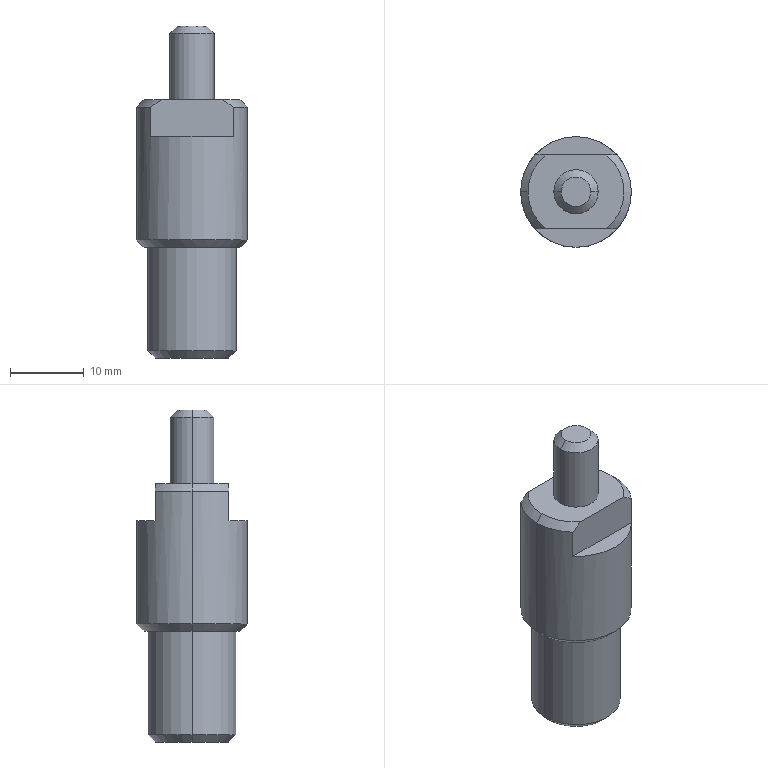Part | SolidWorks | features Chamfer 4, ICE 3, Extrusion 1 | 1 solid | 23 faces | box 15 x 15 x 45 mm | volume 5260 mm3 | cone 9 | plane 8 | cylinder 6 | commonest cylinder face diameters 6 x2 12 x2 15 x2
STEP:
#1=CARTESIAN_POINT('',(-6.5,0.,20.));
#2=VERTEX_POINT('',#1);
#3=CARTESIAN_POINT('',(-4.153,-5.,20.));
#4=VERTEX_POINT('',#3);
#5=CARTESIAN_POINT('',(0.,0.,20.));
#6=DIRECTION('',(0.,0.,1.));
#7=DIRECTION('',(1.,0.,0.));
#8=AXIS2_PLACEMENT_3D('',#5,#6,#7);
#9=CIRCLE('',#8,6.5);
#10=EDGE_CURVE('',#2,#4,#9,.T.);
#11=ORIENTED_EDGE('',*,*,#10,.F.);
#12=CARTESIAN_POINT('',(-7.5,0.,19.));
#13=VERTEX_POINT('',#12);
#14=CARTESIAN_POINT('',(-6.5,0.,20.));
#15=DIRECTION('',(-0.7071,0.,-0.7071));
#16=VECTOR('',#15,1000.);
#17=LINE('',#14,#16);
#18=EDGE_CURVE('',#2,#13,#17,.T.);
#19=ORIENTED_EDGE('',*,*,#18,.T.);
#20=CARTESIAN_POINT('',(-5.59,-5.,19.));
#21=VERTEX_POINT('',#20);
#22=CARTESIAN_POINT('',(0.,0.,19.));
#23=DIRECTION('',(0.,0.,-1.));
#24=DIRECTION('',(1.,0.,0.));
#25=AXIS2_PLACEMENT_3D('',#22,#23,#24);
#26=CIRCLE('',#25,7.5);
#27=EDGE_CURVE('',#21,#13,#26,.T.);
#28=ORIENTED_EDGE('',*,*,#27,.F.);
#29=CARTESIAN_POINT('',(-4.153,-5.,20.));
#30=CARTESIAN_POINT('',(-4.644,-5.,19.687));
#31=CARTESIAN_POINT('',(-5.121,-5.,19.35));
#32=CARTESIAN_POINT('',(-5.59,-5.,19.));
#33=B_SPLINE_CURVE_WITH_KNOTS('',3,(#29,#30,#31,#32),.UNSPECIFIED.,.F.,.F.,(4,4),(0.0243,0.02606),.UNSPECIFIED.);
#34=EDGE_CURVE('',#4,#21,#33,.T.);
#35=ORIENTED_EDGE('',*,*,#34,.F.);
#36=EDGE_LOOP('',(#11,#19,#28,#35));
#37=FACE_OUTER_BOUND('',#36,.T.);
#38=CARTESIAN_POINT('',(0.,0.,20.));
#39=DIRECTION('',(0.,0.,-1.));
#40=DIRECTION('',(-1.,0.,0.));
#41=AXIS2_PLACEMENT_3D('',#38,#39,#40);
#42=CONICAL_SURFACE('',#41,6.5,0.7854);
#43=ADVANCED_FACE('',(#37),#42,.T.);
#44=CARTESIAN_POINT('',(-6.5,0.,0.));
#45=VERTEX_POINT('',#44);
#46=CARTESIAN_POINT('',(6.5,0.,0.));
#47=VERTEX_POINT('',#46);
#48=CARTESIAN_POINT('',(0.,0.,0.));
#49=DIRECTION('',(0.,0.,-1.));
#50=DIRECTION('',(-1.,0.,0.));
#51=AXIS2_PLACEMENT_3D('',#48,#49,#50);
#52=CIRCLE('',#51,6.5);
#53=EDGE_CURVE('',#45,#47,#52,.T.);
#54=ORIENTED_EDGE('',*,*,#53,.F.);
#55=CARTESIAN_POINT('',(-7.5,0.,1.));
#56=VERTEX_POINT('',#55);
#57=CARTESIAN_POINT('',(-6.5,0.,0.));
#58=DIRECTION('',(-0.7071,0.,0.7071));
#59=VECTOR('',#58,1000.);
#60=LINE('',#57,#59);
#61=EDGE_CURVE('',#45,#56,#60,.T.);
#62=ORIENTED_EDGE('',*,*,#61,.T.);
#63=CARTESIAN_POINT('',(7.5,0.,1.));
#64=VERTEX_POINT('',#63);
#65=CARTESIAN_POINT('',(0.,0.,1.));
#66=DIRECTION('',(0.,0.,1.));
#67=DIRECTION('',(-1.,0.,0.));
#68=AXIS2_PLACEMENT_3D('',#65,#66,#67);
#69=CIRCLE('',#68,7.5);
#70=EDGE_CURVE('',#64,#56,#69,.T.);
#71=ORIENTED_EDGE('',*,*,#70,.F.);
#72=CARTESIAN_POINT('',(6.5,0.,0.));
#73=DIRECTION('',(0.7071,0.,0.7071));
#74=VECTOR('',#73,1000.);
#75=LINE('',#72,#74);
#76=EDGE_CURVE('',#47,#64,#75,.T.);
#77=ORIENTED_EDGE('',*,*,#76,.F.);
#78=EDGE_LOOP('',(#54,#62,#71,#77));
#79=FACE_OUTER_BOUND('',#78,.T.);
#80=CARTESIAN_POINT('',(0.,0.,0.));
#81=DIRECTION('',(0.,0.,1.));
#82=DIRECTION('',(1.,0.,0.));
#83=AXIS2_PLACEMENT_3D('',#80,#81,#82);
#84=CONICAL_SURFACE('',#83,6.5,0.7854);
#85=ADVANCED_FACE('',(#79),#84,.T.);
#86=CARTESIAN_POINT('',(-5.,0.,-15.));
#87=VERTEX_POINT('',#86);
#88=CARTESIAN_POINT('',(5.,0.,-15.));
#89=VERTEX_POINT('',#88);
#90=CARTESIAN_POINT('',(0.,0.,-15.));
#91=DIRECTION('',(0.,0.,-1.));
#92=DIRECTION('',(1.,0.,0.));
#93=AXIS2_PLACEMENT_3D('',#90,#91,#92);
#94=CIRCLE('',#93,5.);
#95=EDGE_CURVE('',#87,#89,#94,.T.);
#96=ORIENTED_EDGE('',*,*,#95,.F.);
#97=CARTESIAN_POINT('',(-6.,0.,-14.));
#98=VERTEX_POINT('',#97);
#99=CARTESIAN_POINT('',(-5.,0.,-15.));
#100=DIRECTION('',(-0.7071,0.,0.7071));
#101=VECTOR('',#100,1000.);
#102=LINE('',#99,#101);
#103=EDGE_CURVE('',#87,#98,#102,.T.);
#104=ORIENTED_EDGE('',*,*,#103,.T.);
#105=CARTESIAN_POINT('',(6.,0.,-14.));
#106=VERTEX_POINT('',#105);
#107=CARTESIAN_POINT('',(0.,0.,-14.));
#108=DIRECTION('',(0.,0.,1.));
#109=DIRECTION('',(1.,0.,0.));
#110=AXIS2_PLACEMENT_3D('',#107,#108,#109);
#111=CIRCLE('',#110,6.);
#112=EDGE_CURVE('',#106,#98,#111,.T.);
#113=ORIENTED_EDGE('',*,*,#112,.F.);
#114=CARTESIAN_POINT('',(5.,0.,-15.));
#115=DIRECTION('',(0.7071,0.,0.7071));
#116=VECTOR('',#115,1000.);
#117=LINE('',#114,#116);
#118=EDGE_CURVE('',#89,#106,#117,.T.);
#119=ORIENTED_EDGE('',*,*,#118,.F.);
#120=EDGE_LOOP('',(#96,#104,#113,#119));
#121=FACE_OUTER_BOUND('',#120,.T.);
#122=CARTESIAN_POINT('',(0.,0.,-15.));
#123=DIRECTION('',(0.,0.,1.));
#124=DIRECTION('',(1.,0.,0.));
#125=AXIS2_PLACEMENT_3D('',#122,#123,#124);
#126=CONICAL_SURFACE('',#125,5.,0.7854);
#127=ADVANCED_FACE('',(#121),#126,.T.);
#128=CARTESIAN_POINT('',(-6.,0.,0.));
#129=VERTEX_POINT('',#128);
#130=CARTESIAN_POINT('',(6.,0.,0.));
#131=VERTEX_POINT('',#130);
#132=CARTESIAN_POINT('',(0.,0.,0.));
#133=DIRECTION('',(0.,0.,-1.));
#134=DIRECTION('',(-1.,0.,0.));
#135=AXIS2_PLACEMENT_3D('',#132,#133,#134);
#136=CIRCLE('',#135,6.);
#137=EDGE_CURVE('',#129,#131,#136,.T.);
#138=ORIENTED_EDGE('',*,*,#137,.T.);
#139=CARTESIAN_POINT('',(6.,0.,0.));
#140=DIRECTION('',(0.,0.,-1.));
#141=VECTOR('',#140,1000.);
#142=LINE('',#139,#141);
#143=EDGE_CURVE('',#131,#106,#142,.T.);
#144=ORIENTED_EDGE('',*,*,#143,.T.);
#145=ORIENTED_EDGE('',*,*,#112,.T.);
#146=CARTESIAN_POINT('',(-6.,0.,0.));
#147=DIRECTION('',(0.,0.,-1.));
#148=VECTOR('',#147,1000.);
#149=LINE('',#146,#148);
#150=EDGE_CURVE('',#129,#98,#149,.T.);
#151=ORIENTED_EDGE('',*,*,#150,.F.);
#152=EDGE_LOOP('',(#138,#144,#145,#151));
#153=FACE_OUTER_BOUND('',#152,.T.);
#154=CARTESIAN_POINT('',(0.,0.,0.));
#155=DIRECTION('',(0.,0.,-1.));
#156=DIRECTION('',(-1.,0.,0.));
#157=AXIS2_PLACEMENT_3D('',#154,#155,#156);
#158=CYLINDRICAL_SURFACE('',#157,6.);
#159=ADVANCED_FACE('',(#153),#158,.T.);
#160=CARTESIAN_POINT('',(2.,0.,30.));
#161=VERTEX_POINT('',#160);
#162=CARTESIAN_POINT('',(-2.,0.,30.));
#163=VERTEX_POINT('',#162);
#164=CARTESIAN_POINT('',(0.,0.,30.));
#165=DIRECTION('',(0.,0.,1.));
#166=DIRECTION('',(1.,0.,0.));
#167=AXIS2_PLACEMENT_3D('',#164,#165,#166);
#168=CIRCLE('',#167,2.);
#169=EDGE_CURVE('',#161,#163,#168,.T.);
#170=ORIENTED_EDGE('',*,*,#169,.F.);
#171=CARTESIAN_POINT('',(3.,0.,29.));
#172=VERTEX_POINT('',#171);
#173=CARTESIAN_POINT('',(2.,0.,30.));
#174=DIRECTION('',(0.7071,0.,-0.7071));
#175=VECTOR('',#174,1000.);
#176=LINE('',#173,#175);
#177=EDGE_CURVE('',#161,#172,#176,.T.);
#178=ORIENTED_EDGE('',*,*,#177,.T.);
#179=CARTESIAN_POINT('',(-3.,0.,29.));
#180=VERTEX_POINT('',#179);
#181=CARTESIAN_POINT('',(0.,0.,29.));
#182=DIRECTION('',(0.,0.,-1.));
#183=DIRECTION('',(1.,0.,0.));
#184=AXIS2_PLACEMENT_3D('',#181,#182,#183);
#185=CIRCLE('',#184,3.);
#186=EDGE_CURVE('',#180,#172,#185,.T.);
#187=ORIENTED_EDGE('',*,*,#186,.F.);
#188=CARTESIAN_POINT('',(-2.,0.,30.));
#189=DIRECTION('',(-0.7071,0.,-0.7071));
#190=VECTOR('',#189,1000.);
#191=LINE('',#188,#190);
#192=EDGE_CURVE('',#163,#180,#191,.T.);
#193=ORIENTED_EDGE('',*,*,#192,.F.);
#194=EDGE_LOOP('',(#170,#178,#187,#193));
#195=FACE_OUTER_BOUND('',#194,.T.);
#196=CARTESIAN_POINT('',(0.,0.,30.));
#197=DIRECTION('',(0.,0.,-1.));
#198=DIRECTION('',(-1.,0.,0.));
#199=AXIS2_PLACEMENT_3D('',#196,#197,#198);
#200=CONICAL_SURFACE('',#199,2.,0.7854);
#201=ADVANCED_FACE('',(#195),#200,.T.);
#202=CARTESIAN_POINT('',(3.,0.,20.));
#203=VERTEX_POINT('',#202);
#204=CARTESIAN_POINT('',(-3.,0.,20.));
#205=VERTEX_POINT('',#204);
#206=CARTESIAN_POINT('',(0.,0.,20.));
#207=DIRECTION('',(0.,0.,1.));
#208=DIRECTION('',(1.,0.,0.));
#209=AXIS2_PLACEMENT_3D('',#206,#207,#208);
#210=CIRCLE('',#209,3.);
#211=EDGE_CURVE('',#203,#205,#210,.T.);
#212=ORIENTED_EDGE('',*,*,#211,.T.);
#213=CARTESIAN_POINT('',(-3.,0.,20.));
#214=DIRECTION('',(0.,0.,1.));
#215=VECTOR('',#214,1000.);
#216=LINE('',#213,#215);
#217=EDGE_CURVE('',#205,#180,#216,.T.);
#218=ORIENTED_EDGE('',*,*,#217,.T.);
#219=ORIENTED_EDGE('',*,*,#186,.T.);
#220=CARTESIAN_POINT('',(3.,0.,20.));
#221=DIRECTION('',(0.,0.,1.));
#222=VECTOR('',#221,1000.);
#223=LINE('',#220,#222);
#224=EDGE_CURVE('',#203,#172,#223,.T.);
#225=ORIENTED_EDGE('',*,*,#224,.F.);
#226=EDGE_LOOP('',(#212,#218,#219,#225));
#227=FACE_OUTER_BOUND('',#226,.T.);
#228=CARTESIAN_POINT('',(0.,0.,20.));
#229=DIRECTION('',(0.,0.,1.));
#230=DIRECTION('',(1.,0.,0.));
#231=AXIS2_PLACEMENT_3D('',#228,#229,#230);
#232=CYLINDRICAL_SURFACE('',#231,3.);
#233=ADVANCED_FACE('',(#227),#232,.T.);
#234=ORIENTED_EDGE('',*,*,#70,.T.);
#235=CARTESIAN_POINT('',(-7.5,0.,-15.));
#236=DIRECTION('',(0.,0.,1.));
#237=VECTOR('',#236,1000.);
#238=LINE('',#235,#237);
#239=EDGE_CURVE('',#56,#13,#238,.T.);
#240=ORIENTED_EDGE('',*,*,#239,.T.);
#241=CARTESIAN_POINT('',(-5.59,5.,19.));
#242=VERTEX_POINT('',#241);
#243=CARTESIAN_POINT('',(0.,0.,19.));
#244=DIRECTION('',(0.,0.,-1.));
#245=DIRECTION('',(1.,0.,0.));
#246=AXIS2_PLACEMENT_3D('',#243,#244,#245);
#247=CIRCLE('',#246,7.5);
#248=EDGE_CURVE('',#13,#242,#247,.T.);
#249=ORIENTED_EDGE('',*,*,#248,.T.);
#250=CARTESIAN_POINT('',(-5.59,5.,15.));
#251=VERTEX_POINT('',#250);
#252=CARTESIAN_POINT('',(-5.59,5.,-15.));
#253=DIRECTION('',(0.,0.,1.));
#254=VECTOR('',#253,1000.);
#255=LINE('',#252,#254);
#256=EDGE_CURVE('',#251,#242,#255,.T.);
#257=ORIENTED_EDGE('',*,*,#256,.F.);
#258=CARTESIAN_POINT('',(5.59,5.,15.));
#259=VERTEX_POINT('',#258);
#260=CARTESIAN_POINT('',(0.,0.,15.));
#261=DIRECTION('',(0.,0.,1.));
#262=DIRECTION('',(-1.,0.,0.));
#263=AXIS2_PLACEMENT_3D('',#260,#261,#262);
#264=CIRCLE('',#263,7.5);
#265=EDGE_CURVE('',#259,#251,#264,.T.);
#266=ORIENTED_EDGE('',*,*,#265,.F.);
#267=CARTESIAN_POINT('',(5.59,5.,19.));
#268=VERTEX_POINT('',#267);
#269=CARTESIAN_POINT('',(5.59,5.,-15.));
#270=DIRECTION('',(0.,0.,-1.));
#271=VECTOR('',#270,1000.);
#272=LINE('',#269,#271);
#273=EDGE_CURVE('',#268,#259,#272,.T.);
#274=ORIENTED_EDGE('',*,*,#273,.F.);
#275=CARTESIAN_POINT('',(7.5,0.,19.));
#276=VERTEX_POINT('',#275);
#277=CARTESIAN_POINT('',(0.,0.,19.));
#278=DIRECTION('',(0.,0.,-1.));
#279=DIRECTION('',(1.,0.,0.));
#280=AXIS2_PLACEMENT_3D('',#277,#278,#279);
#281=CIRCLE('',#280,7.5);
#282=EDGE_CURVE('',#268,#276,#281,.T.);
#283=ORIENTED_EDGE('',*,*,#282,.T.);
#284=CARTESIAN_POINT('',(7.5,0.,-15.));
#285=DIRECTION('',(0.,0.,1.));
#286=VECTOR('',#285,1000.);
#287=LINE('',#284,#286);
#288=EDGE_CURVE('',#64,#276,#287,.T.);
#289=ORIENTED_EDGE('',*,*,#288,.F.);
#290=EDGE_LOOP('',(#234,#240,#249,#257,#266,#274,#283,#289));
#291=FACE_OUTER_BOUND('',#290,.T.);
#292=CARTESIAN_POINT('',(0.,0.,-15.));
#293=DIRECTION('',(0.,0.,1.));
#294=DIRECTION('',(1.,0.,0.));
#295=AXIS2_PLACEMENT_3D('',#292,#293,#294);
#296=CYLINDRICAL_SURFACE('',#295,7.5);
#297=ADVANCED_FACE('',(#291),#296,.T.);
#298=CARTESIAN_POINT('',(5.59,-5.,19.));
#299=VERTEX_POINT('',#298);
#300=CARTESIAN_POINT('',(4.153,-5.,20.));
#301=VERTEX_POINT('',#300);
#302=CARTESIAN_POINT('',(5.59,-5.,19.));
#303=CARTESIAN_POINT('',(5.123,-5.,19.348));
#304=CARTESIAN_POINT('',(4.646,-5.,19.685));
#305=CARTESIAN_POINT('',(4.153,-5.,20.));
#306=B_SPLINE_CURVE_WITH_KNOTS('',3,(#302,#303,#304,#305),.UNSPECIFIED.,.F.,.F.,(4,4),(0.01359,0.01534),.UNSPECIFIED.);
#307=EDGE_CURVE('',#299,#301,#306,.T.);
#308=ORIENTED_EDGE('',*,*,#307,.F.);
#309=CARTESIAN_POINT('',(0.,0.,19.));
#310=DIRECTION('',(0.,0.,-1.));
#311=DIRECTION('',(1.,0.,0.));
#312=AXIS2_PLACEMENT_3D('',#309,#310,#311);
#313=CIRCLE('',#312,7.5);
#314=EDGE_CURVE('',#276,#299,#313,.T.);
#315=ORIENTED_EDGE('',*,*,#314,.F.);
#316=ORIENTED_EDGE('',*,*,#282,.F.);
#317=CARTESIAN_POINT('',(4.153,5.,20.));
#318=VERTEX_POINT('',#317);
#319=CARTESIAN_POINT('',(4.153,5.,20.));
#320=CARTESIAN_POINT('',(4.644,5.,19.687));
#321=CARTESIAN_POINT('',(5.121,5.,19.35));
#322=CARTESIAN_POINT('',(5.59,5.,19.));
#323=B_SPLINE_CURVE_WITH_KNOTS('',3,(#319,#320,#321,#322),.UNSPECIFIED.,.F.,.F.,(4,4),(0.0243,0.02606),.UNSPECIFIED.);
#324=EDGE_CURVE('',#318,#268,#323,.T.);
#325=ORIENTED_EDGE('',*,*,#324,.F.);
#326=CARTESIAN_POINT('',(0.,0.,20.));
#327=DIRECTION('',(0.,0.,1.));
#328=DIRECTION('',(1.,0.,0.));
#329=AXIS2_PLACEMENT_3D('',#326,#327,#328);
#330=CIRCLE('',#329,6.5);
#331=EDGE_CURVE('',#301,#318,#330,.T.);
#332=ORIENTED_EDGE('',*,*,#331,.F.);
#333=EDGE_LOOP('',(#308,#315,#316,#325,#332));
#334=FACE_OUTER_BOUND('',#333,.T.);
#335=CARTESIAN_POINT('',(0.,0.,20.));
#336=DIRECTION('',(0.,0.,-1.));
#337=DIRECTION('',(-1.,0.,0.));
#338=AXIS2_PLACEMENT_3D('',#335,#336,#337);
#339=CONICAL_SURFACE('',#338,6.5,0.7854);
#340=ADVANCED_FACE('',(#334),#339,.T.);
#341=ORIENTED_EDGE('',*,*,#239,.F.);
#342=CARTESIAN_POINT('',(0.,0.,1.));
#343=DIRECTION('',(0.,0.,1.));
#344=DIRECTION('',(-1.,0.,0.));
#345=AXIS2_PLACEMENT_3D('',#342,#343,#344);
#346=CIRCLE('',#345,7.5);
#347=EDGE_CURVE('',#56,#64,#346,.T.);
#348=ORIENTED_EDGE('',*,*,#347,.T.);
#349=ORIENTED_EDGE('',*,*,#288,.T.);
#350=ORIENTED_EDGE('',*,*,#314,.T.);
#351=CARTESIAN_POINT('',(5.59,-5.,15.));
#352=VERTEX_POINT('',#351);
#353=CARTESIAN_POINT('',(5.59,-5.,-15.));
#354=DIRECTION('',(0.,0.,1.));
#355=VECTOR('',#354,1000.);
#356=LINE('',#353,#355);
#357=EDGE_CURVE('',#352,#299,#356,.T.);
#358=ORIENTED_EDGE('',*,*,#357,.F.);
#359=CARTESIAN_POINT('',(-5.59,-5.,15.));
#360=VERTEX_POINT('',#359);
#361=CARTESIAN_POINT('',(0.,0.,15.));
#362=DIRECTION('',(0.,0.,-1.));
#363=DIRECTION('',(1.,0.,0.));
#364=AXIS2_PLACEMENT_3D('',#361,#362,#363);
#365=CIRCLE('',#364,7.5);
#366=EDGE_CURVE('',#352,#360,#365,.T.);
#367=ORIENTED_EDGE('',*,*,#366,.T.);
#368=CARTESIAN_POINT('',(-5.59,-5.,-15.));
#369=DIRECTION('',(0.,0.,-1.));
#370=VECTOR('',#369,1000.);
#371=LINE('',#368,#370);
#372=EDGE_CURVE('',#21,#360,#371,.T.);
#373=ORIENTED_EDGE('',*,*,#372,.F.);
#374=ORIENTED_EDGE('',*,*,#27,.T.);
#375=EDGE_LOOP('',(#341,#348,#349,#350,#358,#367,#373,#374));
#376=FACE_OUTER_BOUND('',#375,.T.);
#377=CARTESIAN_POINT('',(0.,0.,-15.));
#378=DIRECTION('',(0.,0.,1.));
#379=DIRECTION('',(1.,0.,0.));
#380=AXIS2_PLACEMENT_3D('',#377,#378,#379);
#381=CYLINDRICAL_SURFACE('',#380,7.5);
#382=ADVANCED_FACE('',(#376),#381,.T.);
#383=CARTESIAN_POINT('',(-14.513,-5.,20.));
#384=DIRECTION('',(-1.,0.,0.));
#385=VECTOR('',#384,1000.);
#386=LINE('',#383,#385);
#387=EDGE_CURVE('',#301,#4,#386,.T.);
#388=ORIENTED_EDGE('',*,*,#387,.F.);
#389=ORIENTED_EDGE('',*,*,#331,.T.);
#390=CARTESIAN_POINT('',(-4.153,5.,20.));
#391=VERTEX_POINT('',#390);
#392=CARTESIAN_POINT('',(-15.452,5.,20.));
#393=DIRECTION('',(1.,0.,0.));
#394=VECTOR('',#393,1000.);
#395=LINE('',#392,#394);
#396=EDGE_CURVE('',#391,#318,#395,.T.);
#397=ORIENTED_EDGE('',*,*,#396,.F.);
#398=CARTESIAN_POINT('',(0.,0.,20.));
#399=DIRECTION('',(0.,0.,1.));
#400=DIRECTION('',(1.,0.,0.));
#401=AXIS2_PLACEMENT_3D('',#398,#399,#400);
#402=CIRCLE('',#401,6.5);
#403=EDGE_CURVE('',#391,#2,#402,.T.);
#404=ORIENTED_EDGE('',*,*,#403,.T.);
#405=ORIENTED_EDGE('',*,*,#10,.T.);
#406=EDGE_LOOP('',(#388,#389,#397,#404,#405));
#407=FACE_OUTER_BOUND('',#406,.T.);
#408=ORIENTED_EDGE('',*,*,#211,.F.);
#409=CARTESIAN_POINT('',(0.,0.,20.));
#410=DIRECTION('',(0.,0.,1.));
#411=DIRECTION('',(1.,0.,0.));
#412=AXIS2_PLACEMENT_3D('',#409,#410,#411);
#413=CIRCLE('',#412,3.);
#414=EDGE_CURVE('',#205,#203,#413,.T.);
#415=ORIENTED_EDGE('',*,*,#414,.F.);
#416=EDGE_LOOP('',(#408,#415));
#417=FACE_BOUND('',#416,.T.);
#418=CARTESIAN_POINT('',(0.,0.,20.));
#419=DIRECTION('',(0.,0.,1.));
#420=DIRECTION('',(1.,0.,0.));
#421=AXIS2_PLACEMENT_3D('',#418,#419,#420);
#422=PLANE('',#421);
#423=ADVANCED_FACE('',(#407,#417),#422,.T.);
#424=ORIENTED_EDGE('',*,*,#217,.F.);
#425=ORIENTED_EDGE('',*,*,#414,.T.);
#426=ORIENTED_EDGE('',*,*,#224,.T.);
#427=CARTESIAN_POINT('',(0.,0.,29.));
#428=DIRECTION('',(0.,0.,-1.));
#429=DIRECTION('',(1.,0.,0.));
#430=AXIS2_PLACEMENT_3D('',#427,#428,#429);
#431=CIRCLE('',#430,3.);
#432=EDGE_CURVE('',#172,#180,#431,.T.);
#433=ORIENTED_EDGE('',*,*,#432,.T.);
#434=EDGE_LOOP('',(#424,#425,#426,#433));
#435=FACE_OUTER_BOUND('',#434,.T.);
#436=CARTESIAN_POINT('',(0.,0.,20.));
#437=DIRECTION('',(0.,0.,1.));
#438=DIRECTION('',(1.,0.,0.));
#439=AXIS2_PLACEMENT_3D('',#436,#437,#438);
#440=CYLINDRICAL_SURFACE('',#439,3.);
#441=ADVANCED_FACE('',(#435),#440,.T.);
#442=CARTESIAN_POINT('',(0.,0.,30.));
#443=DIRECTION('',(0.,0.,1.));
#444=DIRECTION('',(1.,0.,0.));
#445=AXIS2_PLACEMENT_3D('',#442,#443,#444);
#446=CIRCLE('',#445,2.);
#447=EDGE_CURVE('',#163,#161,#446,.T.);
#448=ORIENTED_EDGE('',*,*,#447,.T.);
#449=ORIENTED_EDGE('',*,*,#169,.T.);
#450=EDGE_LOOP('',(#448,#449));
#451=FACE_OUTER_BOUND('',#450,.T.);
#452=CARTESIAN_POINT('',(0.,0.,30.));
#453=DIRECTION('',(0.,0.,1.));
#454=DIRECTION('',(1.,0.,0.));
#455=AXIS2_PLACEMENT_3D('',#452,#453,#454);
#456=PLANE('',#455);
#457=ADVANCED_FACE('',(#451),#456,.T.);
#458=ORIENTED_EDGE('',*,*,#177,.F.);
#459=ORIENTED_EDGE('',*,*,#447,.F.);
#460=ORIENTED_EDGE('',*,*,#192,.T.);
#461=ORIENTED_EDGE('',*,*,#432,.F.);
#462=EDGE_LOOP('',(#458,#459,#460,#461));
#463=FACE_OUTER_BOUND('',#462,.T.);
#464=CARTESIAN_POINT('',(0.,0.,30.));
#465=DIRECTION('',(0.,0.,-1.));
#466=DIRECTION('',(-1.,0.,0.));
#467=AXIS2_PLACEMENT_3D('',#464,#465,#466);
#468=CONICAL_SURFACE('',#467,2.,0.7854);
#469=ADVANCED_FACE('',(#463),#468,.T.);
#470=CARTESIAN_POINT('',(0.,0.,0.));
#471=DIRECTION('',(0.,0.,-1.));
#472=DIRECTION('',(-1.,0.,0.));
#473=AXIS2_PLACEMENT_3D('',#470,#471,#472);
#474=CIRCLE('',#473,6.5);
#475=EDGE_CURVE('',#47,#45,#474,.T.);
#476=ORIENTED_EDGE('',*,*,#475,.T.);
#477=ORIENTED_EDGE('',*,*,#53,.T.);
#478=EDGE_LOOP('',(#476,#477));
#479=FACE_OUTER_BOUND('',#478,.T.);
#480=ORIENTED_EDGE('',*,*,#137,.F.);
#481=CARTESIAN_POINT('',(0.,0.,0.));
#482=DIRECTION('',(0.,0.,-1.));
#483=DIRECTION('',(-1.,0.,0.));
#484=AXIS2_PLACEMENT_3D('',#481,#482,#483);
#485=CIRCLE('',#484,6.);
#486=EDGE_CURVE('',#131,#129,#485,.T.);
#487=ORIENTED_EDGE('',*,*,#486,.F.);
#488=EDGE_LOOP('',(#480,#487));
#489=FACE_BOUND('',#488,.T.);
#490=CARTESIAN_POINT('',(0.,0.,0.));
#491=DIRECTION('',(0.,0.,-1.));
#492=DIRECTION('',(-1.,0.,0.));
#493=AXIS2_PLACEMENT_3D('',#490,#491,#492);
#494=PLANE('',#493);
#495=ADVANCED_FACE('',(#479,#489),#494,.T.);
#496=ORIENTED_EDGE('',*,*,#143,.F.);
#497=ORIENTED_EDGE('',*,*,#486,.T.);
#498=ORIENTED_EDGE('',*,*,#150,.T.);
#499=CARTESIAN_POINT('',(0.,0.,-14.));
#500=DIRECTION('',(0.,0.,1.));
#501=DIRECTION('',(1.,0.,0.));
#502=AXIS2_PLACEMENT_3D('',#499,#500,#501);
#503=CIRCLE('',#502,6.);
#504=EDGE_CURVE('',#98,#106,#503,.T.);
#505=ORIENTED_EDGE('',*,*,#504,.T.);
#506=EDGE_LOOP('',(#496,#497,#498,#505));
#507=FACE_OUTER_BOUND('',#506,.T.);
#508=CARTESIAN_POINT('',(0.,0.,0.));
#509=DIRECTION('',(0.,0.,-1.));
#510=DIRECTION('',(-1.,0.,0.));
#511=AXIS2_PLACEMENT_3D('',#508,#509,#510);
#512=CYLINDRICAL_SURFACE('',#511,6.);
#513=ADVANCED_FACE('',(#507),#512,.T.);
#514=CARTESIAN_POINT('',(0.,0.,-15.));
#515=DIRECTION('',(0.,0.,-1.));
#516=DIRECTION('',(1.,0.,0.));
#517=AXIS2_PLACEMENT_3D('',#514,#515,#516);
#518=CIRCLE('',#517,5.);
#519=EDGE_CURVE('',#89,#87,#518,.T.);
#520=ORIENTED_EDGE('',*,*,#519,.T.);
#521=ORIENTED_EDGE('',*,*,#95,.T.);
#522=EDGE_LOOP('',(#520,#521));
#523=FACE_OUTER_BOUND('',#522,.T.);
#524=CARTESIAN_POINT('',(0.,0.,-15.));
#525=DIRECTION('',(0.,0.,1.));
#526=DIRECTION('',(1.,0.,0.));
#527=AXIS2_PLACEMENT_3D('',#524,#525,#526);
#528=PLANE('',#527);
#529=ADVANCED_FACE('',(#523),#528,.F.);
#530=ORIENTED_EDGE('',*,*,#103,.F.);
#531=ORIENTED_EDGE('',*,*,#519,.F.);
#532=ORIENTED_EDGE('',*,*,#118,.T.);
#533=ORIENTED_EDGE('',*,*,#504,.F.);
#534=EDGE_LOOP('',(#530,#531,#532,#533));
#535=FACE_OUTER_BOUND('',#534,.T.);
#536=CARTESIAN_POINT('',(0.,0.,-15.));
#537=DIRECTION('',(0.,0.,1.));
#538=DIRECTION('',(1.,0.,0.));
#539=AXIS2_PLACEMENT_3D('',#536,#537,#538);
#540=CONICAL_SURFACE('',#539,5.,0.7854);
#541=ADVANCED_FACE('',(#535),#540,.T.);
#542=ORIENTED_EDGE('',*,*,#61,.F.);
#543=ORIENTED_EDGE('',*,*,#475,.F.);
#544=ORIENTED_EDGE('',*,*,#76,.T.);
#545=ORIENTED_EDGE('',*,*,#347,.F.);
#546=EDGE_LOOP('',(#542,#543,#544,#545));
#547=FACE_OUTER_BOUND('',#546,.T.);
#548=CARTESIAN_POINT('',(0.,0.,0.));
#549=DIRECTION('',(0.,0.,1.));
#550=DIRECTION('',(1.,0.,0.));
#551=AXIS2_PLACEMENT_3D('',#548,#549,#550);
#552=CONICAL_SURFACE('',#551,6.5,0.7854);
#553=ADVANCED_FACE('',(#547),#552,.T.);
#554=ORIENTED_EDGE('',*,*,#18,.F.);
#555=ORIENTED_EDGE('',*,*,#403,.F.);
#556=CARTESIAN_POINT('',(-5.59,5.,19.));
#557=CARTESIAN_POINT('',(-5.123,5.,19.348));
#558=CARTESIAN_POINT('',(-4.646,5.,19.685));
#559=CARTESIAN_POINT('',(-4.153,5.,20.));
#560=B_SPLINE_CURVE_WITH_KNOTS('',3,(#556,#557,#558,#559),.UNSPECIFIED.,.F.,.F.,(4,4),(0.01359,0.01534),.UNSPECIFIED.);
#561=EDGE_CURVE('',#242,#391,#560,.T.);
#562=ORIENTED_EDGE('',*,*,#561,.F.);
#563=ORIENTED_EDGE('',*,*,#248,.F.);
#564=EDGE_LOOP('',(#554,#555,#562,#563));
#565=FACE_OUTER_BOUND('',#564,.T.);
#566=CARTESIAN_POINT('',(0.,0.,20.));
#567=DIRECTION('',(0.,0.,-1.));
#568=DIRECTION('',(-1.,0.,0.));
#569=AXIS2_PLACEMENT_3D('',#566,#567,#568);
#570=CONICAL_SURFACE('',#569,6.5,0.7854);
#571=ADVANCED_FACE('',(#565),#570,.T.);
#572=ORIENTED_EDGE('',*,*,#256,.T.);
#573=ORIENTED_EDGE('',*,*,#561,.T.);
#574=ORIENTED_EDGE('',*,*,#396,.T.);
#575=ORIENTED_EDGE('',*,*,#324,.T.);
#576=ORIENTED_EDGE('',*,*,#273,.T.);
#577=CARTESIAN_POINT('',(-15.452,5.,15.));
#578=DIRECTION('',(1.,0.,0.));
#579=VECTOR('',#578,1000.);
#580=LINE('',#577,#579);
#581=EDGE_CURVE('',#251,#259,#580,.T.);
#582=ORIENTED_EDGE('',*,*,#581,.F.);
#583=EDGE_LOOP('',(#572,#573,#574,#575,#576,#582));
#584=FACE_OUTER_BOUND('',#583,.T.);
#585=CARTESIAN_POINT('',(-15.452,5.,15.));
#586=DIRECTION('',(0.,-1.,0.));
#587=DIRECTION('',(0.,0.,-1.));
#588=AXIS2_PLACEMENT_3D('',#585,#586,#587);
#589=PLANE('',#588);
#590=ADVANCED_FACE('',(#584),#589,.F.);
#591=ORIENTED_EDGE('',*,*,#265,.T.);
#592=ORIENTED_EDGE('',*,*,#581,.T.);
#593=EDGE_LOOP('',(#591,#592));
#594=FACE_OUTER_BOUND('',#593,.T.);
#595=CARTESIAN_POINT('',(0.,0.,15.));
#596=DIRECTION('',(0.,0.,-1.));
#597=DIRECTION('',(-1.,0.,0.));
#598=AXIS2_PLACEMENT_3D('',#595,#596,#597);
#599=PLANE('',#598);
#600=ADVANCED_FACE('',(#594),#599,.F.);
#601=ORIENTED_EDGE('',*,*,#357,.T.);
#602=ORIENTED_EDGE('',*,*,#307,.T.);
#603=ORIENTED_EDGE('',*,*,#387,.T.);
#604=ORIENTED_EDGE('',*,*,#34,.T.);
#605=ORIENTED_EDGE('',*,*,#372,.T.);
#606=CARTESIAN_POINT('',(-14.513,-5.,15.));
#607=DIRECTION('',(-1.,0.,0.));
#608=VECTOR('',#607,1000.);
#609=LINE('',#606,#608);
#610=EDGE_CURVE('',#352,#360,#609,.T.);
#611=ORIENTED_EDGE('',*,*,#610,.F.);
#612=EDGE_LOOP('',(#601,#602,#603,#604,#605,#611));
#613=FACE_OUTER_BOUND('',#612,.T.);
#614=CARTESIAN_POINT('',(-14.513,-5.,15.));
#615=DIRECTION('',(0.,1.,0.));
#616=DIRECTION('',(0.,0.,1.));
#617=AXIS2_PLACEMENT_3D('',#614,#615,#616);
#618=PLANE('',#617);
#619=ADVANCED_FACE('',(#613),#618,.F.);
#620=ORIENTED_EDGE('',*,*,#610,.T.);
#621=ORIENTED_EDGE('',*,*,#366,.F.);
#622=EDGE_LOOP('',(#620,#621));
#623=FACE_OUTER_BOUND('',#622,.T.);
#624=CARTESIAN_POINT('',(0.,0.,15.));
#625=DIRECTION('',(0.,0.,1.));
#626=DIRECTION('',(1.,0.,0.));
#627=AXIS2_PLACEMENT_3D('',#624,#625,#626);
#628=PLANE('',#627);
#629=ADVANCED_FACE('',(#623),#628,.T.);
#630=CLOSED_SHELL('',(#43,#85,#127,#159,#201,#233,#297,#340,#382,#423,#441,#457,#469,#495,#513,#529,#541,#553,#571,#590,#600,#619,#629));
#631=MANIFOLD_SOLID_BREP('',#630);
#632=CARTESIAN_POINT('',(0.,0.,0.));
#633=DIRECTION('',(0.,0.,1.));
#634=DIRECTION('',(1.,0.,0.));
#635=AXIS2_PLACEMENT_3D('',#632,#633,#634);
#636=(LENGTH_UNIT()NAMED_UNIT(*)SI_UNIT(.MILLI.,.METRE.));
#637=UNCERTAINTY_MEASURE_WITH_UNIT(LENGTH_MEASURE(0.00001),#636,'','');
#638=(NAMED_UNIT(*)PLANE_ANGLE_UNIT()SI_UNIT($,.RADIAN.));
#639=(NAMED_UNIT(*)SI_UNIT($,.STERADIAN.)SOLID_ANGLE_UNIT());
#640=(GEOMETRIC_REPRESENTATION_CONTEXT(3)GLOBAL_UNCERTAINTY_ASSIGNED_CONTEXT((#637))GLOBAL_UNIT_ASSIGNED_CONTEXT((#636,#638,#639))REPRESENTATION_CONTEXT('',''));
#641=ADVANCED_BREP_SHAPE_REPRESENTATION('',(#631,#635),#640);